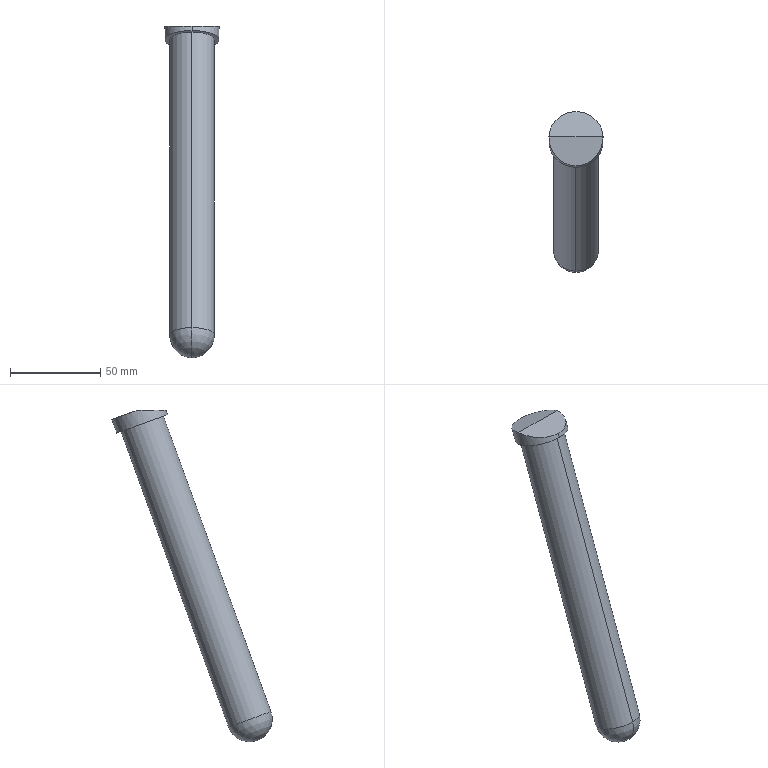Part | Creo | 1 solid | 9 faces | box 30 x 89.014 x 183.975 mm | volume 94577 mm3 | cylinder 4 | plane 3 | sphere 2 | commonest cylinder face diameters 25 x2 30 x2
STEP:
#1=CARTESIAN_POINT('',(0.,-323.2,37.631));
#2=VERTEX_POINT('',#1);
#3=CARTESIAN_POINT('',(0.,-295.009,27.371));
#4=VERTEX_POINT('',#3);
#5=CARTESIAN_POINT('',(0.,-309.104,32.501));
#6=DIRECTION('',(0.,-0.342,-0.9397));
#7=DIRECTION('',(0.,-0.9397,0.342));
#8=AXIS2_PLACEMENT_3D('',#5,#6,#7);
#9=CIRCLE('',#8,15.);
#10=EDGE_CURVE('',#2,#4,#9,.T.);
#11=ORIENTED_EDGE('',*,*,#10,.T.);
#12=CARTESIAN_POINT('',(-0.000000001,-292.273,34.888));
#13=VERTEX_POINT('',#12);
#14=CARTESIAN_POINT('',(-0.000000001,-292.273,34.888));
#15=DIRECTION('',(0.,-0.342,-0.9397));
#16=VECTOR('',#15,8.);
#17=LINE('',#14,#16);
#18=EDGE_CURVE('',#13,#4,#17,.T.);
#19=ORIENTED_EDGE('',*,*,#18,.F.);
#20=CARTESIAN_POINT('',(-15.,-306.317,40.));
#21=VERTEX_POINT('',#20);
#22=CARTESIAN_POINT('',(0.,-306.368,40.019));
#23=DIRECTION('',(0.,0.342,0.9397));
#24=DIRECTION('',(0.,0.9397,-0.342));
#25=AXIS2_PLACEMENT_3D('',#22,#23,#24);
#26=CIRCLE('',#25,15.);
#27=EDGE_CURVE('',#13,#21,#26,.T.);
#28=ORIENTED_EDGE('',*,*,#27,.T.);
#29=CARTESIAN_POINT('',(0.000000025,-322.337,40.));
#30=VERTEX_POINT('',#29);
#31=CARTESIAN_POINT('',(0.000000025,-322.337,40.));
#32=CARTESIAN_POINT('',(-0.9596,-322.337,40.));
#33=CARTESIAN_POINT('',(-2.849,-322.146,40.));
#34=CARTESIAN_POINT('',(-5.649,-321.273,40.));
#35=CARTESIAN_POINT('',(-8.255,-319.822,40.));
#36=CARTESIAN_POINT('',(-10.518,-317.898,40.));
#37=CARTESIAN_POINT('',(-12.451,-315.464,40.));
#38=CARTESIAN_POINT('',(-13.887,-312.683,40.));
#39=CARTESIAN_POINT('',(-14.793,-309.61,40.));
#40=CARTESIAN_POINT('',(-15.004,-307.439,40.));
#41=CARTESIAN_POINT('',(-15.,-306.317,40.));
#42=B_SPLINE_CURVE_WITH_KNOTS('',3,(#31,#32,#33,#34,#35,#36,#37,#38,#39,#40,#41),.UNSPECIFIED.,.F.,.F.,(4,1,1,1,1,1,1,1,4),(0.,0.125,0.25,0.375,0.5,0.625,0.75,0.875,1.),.UNSPECIFIED.);
#43=EDGE_CURVE('',#30,#21,#42,.T.);
#44=ORIENTED_EDGE('',*,*,#43,.F.);
#45=CARTESIAN_POINT('',(0.000000025,-322.337,40.));
#46=DIRECTION('',(-0.00000001,-0.342,-0.9397));
#47=VECTOR('',#46,2.521);
#48=LINE('',#45,#47);
#49=EDGE_CURVE('',#30,#2,#48,.T.);
#50=ORIENTED_EDGE('',*,*,#49,.T.);
#51=EDGE_LOOP('',(#11,#19,#28,#44,#50));
#52=FACE_OUTER_BOUND('',#51,.F.);
#53=CARTESIAN_POINT('',(0.,-302.52,50.59));
#54=DIRECTION('',(0.,-0.342,-0.9397));
#55=DIRECTION('',(0.,-0.9397,0.342));
#56=AXIS2_PLACEMENT_3D('',#53,#54,#55);
#57=CYLINDRICAL_SURFACE('',#56,15.);
#58=ADVANCED_FACE('',(#52),#57,.T.);
#59=CARTESIAN_POINT('',(0.,-309.104,32.501));
#60=DIRECTION('',(0.,-0.342,-0.9397));
#61=DIRECTION('',(0.,0.9397,-0.342));
#62=AXIS2_PLACEMENT_3D('',#59,#60,#61);
#63=CIRCLE('',#62,15.);
#64=EDGE_CURVE('',#4,#2,#63,.T.);
#65=ORIENTED_EDGE('',*,*,#64,.F.);
#66=ORIENTED_EDGE('',*,*,#10,.F.);
#67=EDGE_LOOP('',(#65,#66));
#68=FACE_OUTER_BOUND('',#67,.F.);
#69=CARTESIAN_POINT('',(0.,-297.358,28.226));
#70=VERTEX_POINT('',#69);
#71=CARTESIAN_POINT('',(0.,-320.85,36.776));
#72=VERTEX_POINT('',#71);
#73=CARTESIAN_POINT('',(0.,-309.104,32.501));
#74=DIRECTION('',(0.,0.342,0.9397));
#75=DIRECTION('',(0.,0.9397,-0.342));
#76=AXIS2_PLACEMENT_3D('',#73,#74,#75);
#77=CIRCLE('',#76,12.5);
#78=EDGE_CURVE('',#70,#72,#77,.T.);
#79=ORIENTED_EDGE('',*,*,#78,.F.);
#80=CARTESIAN_POINT('',(0.,-309.104,32.501));
#81=DIRECTION('',(0.,0.342,0.9397));
#82=DIRECTION('',(0.,-0.9397,0.342));
#83=AXIS2_PLACEMENT_3D('',#80,#81,#82);
#84=CIRCLE('',#83,12.5);
#85=EDGE_CURVE('',#72,#70,#84,.T.);
#86=ORIENTED_EDGE('',*,*,#85,.F.);
#87=EDGE_LOOP('',(#79,#86));
#88=FACE_BOUND('',#87,.F.);
#89=CARTESIAN_POINT('',(0.,-309.104,32.501));
#90=DIRECTION('',(0.,-0.342,-0.9397));
#91=DIRECTION('',(0.,-0.9397,0.342));
#92=AXIS2_PLACEMENT_3D('',#89,#90,#91);
#93=PLANE('',#92);
#94=ADVANCED_FACE('',(#68,#88),#93,.T.);
#95=ORIENTED_EDGE('',*,*,#78,.T.);
#96=CARTESIAN_POINT('',(0.,-380.533,-127.2));
#97=VERTEX_POINT('',#96);
#98=CARTESIAN_POINT('',(0.,-320.85,36.776));
#99=DIRECTION('',(0.,-0.342,-0.9397));
#100=VECTOR('',#99,174.5);
#101=LINE('',#98,#100);
#102=EDGE_CURVE('',#72,#97,#101,.T.);
#103=ORIENTED_EDGE('',*,*,#102,.T.);
#104=CARTESIAN_POINT('',(0.,-357.041,-135.751));
#105=VERTEX_POINT('',#104);
#106=CARTESIAN_POINT('',(0.,-368.787,-131.475));
#107=DIRECTION('',(0.,-0.342,-0.9397));
#108=DIRECTION('',(0.,-0.9397,0.342));
#109=AXIS2_PLACEMENT_3D('',#106,#107,#108);
#110=CIRCLE('',#109,12.5);
#111=EDGE_CURVE('',#97,#105,#110,.T.);
#112=ORIENTED_EDGE('',*,*,#111,.T.);
#113=CARTESIAN_POINT('',(0.,-297.358,28.226));
#114=DIRECTION('',(0.,-0.342,-0.9397));
#115=VECTOR('',#114,174.5);
#116=LINE('',#113,#115);
#117=EDGE_CURVE('',#70,#105,#116,.T.);
#118=ORIENTED_EDGE('',*,*,#117,.F.);
#119=EDGE_LOOP('',(#95,#103,#112,#118));
#120=FACE_OUTER_BOUND('',#119,.F.);
#121=CARTESIAN_POINT('',(0.,-286.514,94.568));
#122=DIRECTION('',(0.,-0.342,-0.9397));
#123=DIRECTION('',(0.,-0.9397,0.342));
#124=AXIS2_PLACEMENT_3D('',#121,#122,#123);
#125=CYLINDRICAL_SURFACE('',#124,12.5);
#126=ADVANCED_FACE('',(#120),#125,.T.);
#127=ORIENTED_EDGE('',*,*,#85,.T.);
#128=ORIENTED_EDGE('',*,*,#117,.T.);
#129=CARTESIAN_POINT('',(0.,-368.787,-131.475));
#130=DIRECTION('',(0.,-0.342,-0.9397));
#131=DIRECTION('',(0.,0.9397,-0.342));
#132=AXIS2_PLACEMENT_3D('',#129,#130,#131);
#133=CIRCLE('',#132,12.5);
#134=EDGE_CURVE('',#105,#97,#133,.T.);
#135=ORIENTED_EDGE('',*,*,#134,.T.);
#136=ORIENTED_EDGE('',*,*,#102,.F.);
#137=EDGE_LOOP('',(#127,#128,#135,#136));
#138=FACE_OUTER_BOUND('',#137,.F.);
#139=CARTESIAN_POINT('',(0.,-286.514,94.568));
#140=DIRECTION('',(0.,-0.342,-0.9397));
#141=DIRECTION('',(0.,-0.9397,0.342));
#142=AXIS2_PLACEMENT_3D('',#139,#140,#141);
#143=CYLINDRICAL_SURFACE('',#142,12.5);
#144=ADVANCED_FACE('',(#138),#143,.T.);
#145=ORIENTED_EDGE('',*,*,#134,.F.);
#146=CARTESIAN_POINT('',(0.,-373.062,-143.221));
#147=VERTEX_POINT('',#146);
#148=CARTESIAN_POINT('',(0.,-368.787,-131.475));
#149=DIRECTION('',(-1.,0.,0.));
#150=DIRECTION('',(0.,0.9397,-0.342));
#151=AXIS2_PLACEMENT_3D('',#148,#149,#150);
#152=CIRCLE('',#151,12.5);
#153=EDGE_CURVE('',#105,#147,#152,.T.);
#154=ORIENTED_EDGE('',*,*,#153,.T.);
#155=CARTESIAN_POINT('',(0.,-368.787,-131.475));
#156=DIRECTION('',(1.,0.,0.));
#157=DIRECTION('',(0.,-0.9397,0.342));
#158=AXIS2_PLACEMENT_3D('',#155,#156,#157);
#159=CIRCLE('',#158,12.5);
#160=EDGE_CURVE('',#97,#147,#159,.T.);
#161=ORIENTED_EDGE('',*,*,#160,.F.);
#162=EDGE_LOOP('',(#145,#154,#161));
#163=FACE_OUTER_BOUND('',#162,.F.);
#164=CARTESIAN_POINT('',(0.,-368.787,-131.475));
#165=DIRECTION('',(0.,-0.342,-0.9397));
#166=DIRECTION('',(0.,-0.9397,0.342));
#167=AXIS2_PLACEMENT_3D('',#164,#165,#166);
#168=SPHERICAL_SURFACE('',#167,12.5);
#169=ADVANCED_FACE('',(#163),#168,.T.);
#170=ORIENTED_EDGE('',*,*,#111,.F.);
#171=ORIENTED_EDGE('',*,*,#160,.T.);
#172=ORIENTED_EDGE('',*,*,#153,.F.);
#173=EDGE_LOOP('',(#170,#171,#172));
#174=FACE_OUTER_BOUND('',#173,.F.);
#175=CARTESIAN_POINT('',(0.,-368.787,-131.475));
#176=DIRECTION('',(0.,-0.342,-0.9397));
#177=DIRECTION('',(0.,-0.9397,0.342));
#178=AXIS2_PLACEMENT_3D('',#175,#176,#177);
#179=SPHERICAL_SURFACE('',#178,12.5);
#180=ADVANCED_FACE('',(#174),#179,.T.);
#181=ORIENTED_EDGE('',*,*,#64,.T.);
#182=ORIENTED_EDGE('',*,*,#49,.F.);
#183=CARTESIAN_POINT('',(15.,-306.317,40.));
#184=VERTEX_POINT('',#183);
#185=CARTESIAN_POINT('',(0.000000025,-322.337,40.));
#186=CARTESIAN_POINT('',(0.8648,-322.337,40.));
#187=CARTESIAN_POINT('',(2.562,-322.18,40.));
#188=CARTESIAN_POINT('',(5.024,-321.497,40.));
#189=CARTESIAN_POINT('',(7.355,-320.377,40.));
#190=CARTESIAN_POINT('',(9.511,-318.822,40.));
#191=CARTESIAN_POINT('',(11.395,-316.879,40.));
#192=CARTESIAN_POINT('',(12.942,-314.607,40.));
#193=CARTESIAN_POINT('',(14.111,-312.038,40.));
#194=CARTESIAN_POINT('',(14.84,-309.241,40.));
#195=CARTESIAN_POINT('',(15.003,-307.308,40.));
#196=CARTESIAN_POINT('',(15.,-306.317,40.));
#197=B_SPLINE_CURVE_WITH_KNOTS('',3,(#185,#186,#187,#188,#189,#190,#191,#192,#193,#194,#195,#196),.UNSPECIFIED.,.F.,.F.,(4,1,1,1,1,1,1,1,1,4),(0.,0.1111,0.2222,0.3333,0.4444,0.5556,0.6667,0.7778,0.8889,1.),.UNSPECIFIED.);
#198=EDGE_CURVE('',#30,#184,#197,.T.);
#199=ORIENTED_EDGE('',*,*,#198,.T.);
#200=CARTESIAN_POINT('',(0.,-306.368,40.019));
#201=DIRECTION('',(0.,0.342,0.9397));
#202=DIRECTION('',(1.,0.003409,-0.001241));
#203=AXIS2_PLACEMENT_3D('',#200,#201,#202);
#204=CIRCLE('',#203,15.);
#205=EDGE_CURVE('',#184,#13,#204,.T.);
#206=ORIENTED_EDGE('',*,*,#205,.T.);
#207=ORIENTED_EDGE('',*,*,#18,.T.);
#208=EDGE_LOOP('',(#181,#182,#199,#206,#207));
#209=FACE_OUTER_BOUND('',#208,.F.);
#210=CARTESIAN_POINT('',(0.,-302.52,50.59));
#211=DIRECTION('',(0.,-0.342,-0.9397));
#212=DIRECTION('',(0.,-0.9397,0.342));
#213=AXIS2_PLACEMENT_3D('',#210,#211,#212);
#214=CYLINDRICAL_SURFACE('',#213,15.);
#215=ADVANCED_FACE('',(#209),#214,.T.);
#216=ORIENTED_EDGE('',*,*,#198,.F.);
#217=ORIENTED_EDGE('',*,*,#43,.T.);
#218=CARTESIAN_POINT('',(15.,-306.317,40.));
#219=DIRECTION('',(-1.,0.,0.));
#220=VECTOR('',#219,30.);
#221=LINE('',#218,#220);
#222=EDGE_CURVE('',#184,#21,#221,.T.);
#223=ORIENTED_EDGE('',*,*,#222,.F.);
#224=EDGE_LOOP('',(#216,#217,#223));
#225=FACE_OUTER_BOUND('',#224,.F.);
#226=CARTESIAN_POINT('',(365.934,-307.397,40.));
#227=DIRECTION('',(0.,0.,1.));
#228=DIRECTION('',(-1.,0.,0.));
#229=AXIS2_PLACEMENT_3D('',#226,#227,#228);
#230=PLANE('',#229);
#231=ADVANCED_FACE('',(#225),#230,.T.);
#232=ORIENTED_EDGE('',*,*,#27,.F.);
#233=ORIENTED_EDGE('',*,*,#205,.F.);
#234=ORIENTED_EDGE('',*,*,#222,.T.);
#235=EDGE_LOOP('',(#232,#233,#234));
#236=FACE_OUTER_BOUND('',#235,.F.);
#237=CARTESIAN_POINT('',(0.,-306.368,40.019));
#238=DIRECTION('',(0.,-0.342,-0.9397));
#239=DIRECTION('',(0.,-0.9397,0.342));
#240=AXIS2_PLACEMENT_3D('',#237,#238,#239);
#241=PLANE('',#240);
#242=ADVANCED_FACE('',(#236),#241,.F.);
#243=CLOSED_SHELL('',(#58,#94,#126,#144,#169,#180,#215,#231,#242));
#244=MANIFOLD_SOLID_BREP('',#243);
#245=(LENGTH_UNIT()NAMED_UNIT(*)SI_UNIT(.MILLI.,.METRE.));
#246=UNCERTAINTY_MEASURE_WITH_UNIT(LENGTH_MEASURE(0.02112),#245,'','');
#247=(NAMED_UNIT(*)PLANE_ANGLE_UNIT()SI_UNIT($,.RADIAN.));
#248=PLANE_ANGLE_MEASURE_WITH_UNIT(PLANE_ANGLE_MEASURE(0.01745),#247);
#249=(CONVERSION_BASED_UNIT('DEGREE',#248)NAMED_UNIT(*)PLANE_ANGLE_UNIT());
#250=(NAMED_UNIT(*)SI_UNIT($,.STERADIAN.)SOLID_ANGLE_UNIT());
#251=(GEOMETRIC_REPRESENTATION_CONTEXT(3)GLOBAL_UNCERTAINTY_ASSIGNED_CONTEXT((#246))GLOBAL_UNIT_ASSIGNED_CONTEXT((#245,#249,#250))REPRESENTATION_CONTEXT('',''));
#252=ADVANCED_BREP_SHAPE_REPRESENTATION('',(#244),#251);